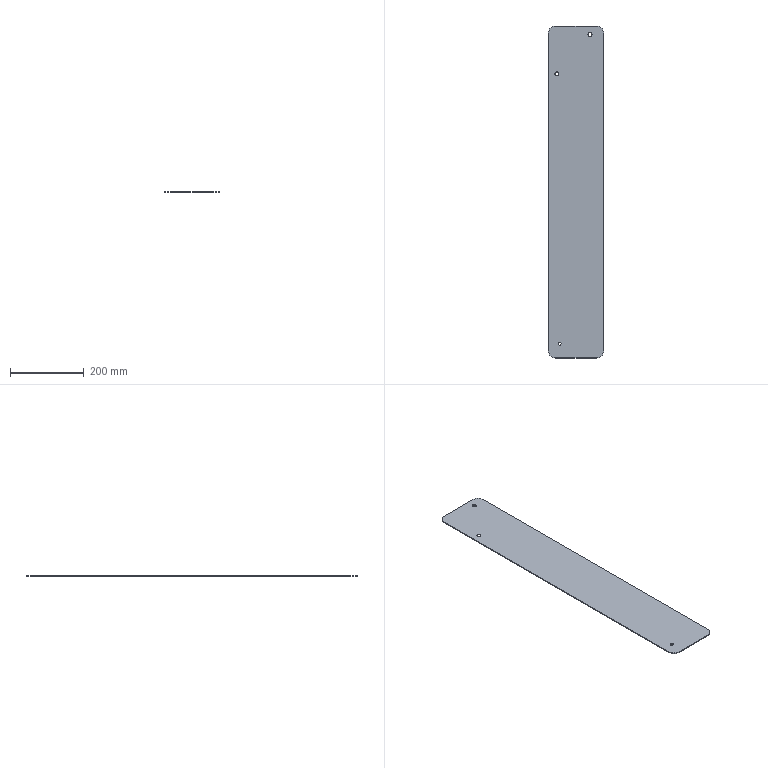Part | SolidWorks | features FlatPattern 1, SMBaseFlange 1, SheetMetal 1 | 1 solid | 16 faces | box 150 x 900 x 2.3 mm | volume 309143 mm3 | cylinder 10 | plane 6 | commonest cylinder face diameters 11 x4 40 x4 8.5 x2
STEP:
#1=CARTESIAN_POINT('',(55.5,-23.,2.3));
#2=VERTEX_POINT('',#1);
#3=CARTESIAN_POINT('',(66.5,-23.,2.3));
#4=VERTEX_POINT('',#3);
#5=CARTESIAN_POINT('',(61.,-23.,2.3));
#6=DIRECTION('',(0.,0.,1.));
#7=DIRECTION('',(1.,0.,0.));
#8=AXIS2_PLACEMENT_3D('',#5,#6,#7);
#9=CIRCLE('',#8,5.5);
#10=EDGE_CURVE('',#2,#4,#9,.T.);
#11=ORIENTED_EDGE('',*,*,#10,.T.);
#12=CARTESIAN_POINT('',(66.5,-23.,0.));
#13=VERTEX_POINT('',#12);
#14=CARTESIAN_POINT('',(66.5,-23.,2.3));
#15=DIRECTION('',(0.,0.,-1.));
#16=VECTOR('',#15,1000.);
#17=LINE('',#14,#16);
#18=EDGE_CURVE('',#4,#13,#17,.T.);
#19=ORIENTED_EDGE('',*,*,#18,.T.);
#20=CARTESIAN_POINT('',(55.5,-23.,0.));
#21=VERTEX_POINT('',#20);
#22=CARTESIAN_POINT('',(61.,-23.,0.));
#23=DIRECTION('',(0.,0.,1.));
#24=DIRECTION('',(1.,0.,0.));
#25=AXIS2_PLACEMENT_3D('',#22,#23,#24);
#26=CIRCLE('',#25,5.5);
#27=EDGE_CURVE('',#21,#13,#26,.T.);
#28=ORIENTED_EDGE('',*,*,#27,.F.);
#29=CARTESIAN_POINT('',(55.5,-23.,2.3));
#30=DIRECTION('',(0.,0.,-1.));
#31=VECTOR('',#30,1000.);
#32=LINE('',#29,#31);
#33=EDGE_CURVE('',#2,#21,#32,.T.);
#34=ORIENTED_EDGE('',*,*,#33,.F.);
#35=EDGE_LOOP('',(#11,#19,#28,#34));
#36=FACE_OUTER_BOUND('',#35,.T.);
#37=CARTESIAN_POINT('',(61.,-23.,2.3));
#38=DIRECTION('',(0.,0.,-1.));
#39=DIRECTION('',(-1.,0.,0.));
#40=AXIS2_PLACEMENT_3D('',#37,#38,#39);
#41=CYLINDRICAL_SURFACE('',#40,5.5);
#42=ADVANCED_FACE('',(#36),#41,.F.);
#43=CARTESIAN_POINT('',(-34.5,-130.,2.3));
#44=VERTEX_POINT('',#43);
#45=CARTESIAN_POINT('',(-23.5,-130.,2.3));
#46=VERTEX_POINT('',#45);
#47=CARTESIAN_POINT('',(-29.,-130.,2.3));
#48=DIRECTION('',(0.,0.,1.));
#49=DIRECTION('',(1.,0.,0.));
#50=AXIS2_PLACEMENT_3D('',#47,#48,#49);
#51=CIRCLE('',#50,5.5);
#52=EDGE_CURVE('',#44,#46,#51,.T.);
#53=ORIENTED_EDGE('',*,*,#52,.T.);
#54=CARTESIAN_POINT('',(-23.5,-130.,0.));
#55=VERTEX_POINT('',#54);
#56=CARTESIAN_POINT('',(-23.5,-130.,2.3));
#57=DIRECTION('',(0.,0.,-1.));
#58=VECTOR('',#57,1000.);
#59=LINE('',#56,#58);
#60=EDGE_CURVE('',#46,#55,#59,.T.);
#61=ORIENTED_EDGE('',*,*,#60,.T.);
#62=CARTESIAN_POINT('',(-34.5,-130.,0.));
#63=VERTEX_POINT('',#62);
#64=CARTESIAN_POINT('',(-29.,-130.,0.));
#65=DIRECTION('',(0.,0.,1.));
#66=DIRECTION('',(1.,0.,0.));
#67=AXIS2_PLACEMENT_3D('',#64,#65,#66);
#68=CIRCLE('',#67,5.5);
#69=EDGE_CURVE('',#63,#55,#68,.T.);
#70=ORIENTED_EDGE('',*,*,#69,.F.);
#71=CARTESIAN_POINT('',(-34.5,-130.,2.3));
#72=DIRECTION('',(0.,0.,-1.));
#73=VECTOR('',#72,1000.);
#74=LINE('',#71,#73);
#75=EDGE_CURVE('',#44,#63,#74,.T.);
#76=ORIENTED_EDGE('',*,*,#75,.F.);
#77=EDGE_LOOP('',(#53,#61,#70,#76));
#78=FACE_OUTER_BOUND('',#77,.T.);
#79=CARTESIAN_POINT('',(-29.,-130.,2.3));
#80=DIRECTION('',(0.,0.,-1.));
#81=DIRECTION('',(-1.,0.,0.));
#82=AXIS2_PLACEMENT_3D('',#79,#80,#81);
#83=CYLINDRICAL_SURFACE('',#82,5.5);
#84=ADVANCED_FACE('',(#78),#83,.F.);
#85=CARTESIAN_POINT('',(-25.75,-861.,2.3));
#86=VERTEX_POINT('',#85);
#87=CARTESIAN_POINT('',(-17.25,-861.,2.3));
#88=VERTEX_POINT('',#87);
#89=CARTESIAN_POINT('',(-21.5,-861.,2.3));
#90=DIRECTION('',(0.,0.,1.));
#91=DIRECTION('',(1.,0.,0.));
#92=AXIS2_PLACEMENT_3D('',#89,#90,#91);
#93=CIRCLE('',#92,4.25);
#94=EDGE_CURVE('',#86,#88,#93,.T.);
#95=ORIENTED_EDGE('',*,*,#94,.T.);
#96=CARTESIAN_POINT('',(-17.25,-861.,0.));
#97=VERTEX_POINT('',#96);
#98=CARTESIAN_POINT('',(-17.25,-861.,2.3));
#99=DIRECTION('',(0.,0.,-1.));
#100=VECTOR('',#99,1000.);
#101=LINE('',#98,#100);
#102=EDGE_CURVE('',#88,#97,#101,.T.);
#103=ORIENTED_EDGE('',*,*,#102,.T.);
#104=CARTESIAN_POINT('',(-25.75,-861.,0.));
#105=VERTEX_POINT('',#104);
#106=CARTESIAN_POINT('',(-21.5,-861.,0.));
#107=DIRECTION('',(0.,0.,1.));
#108=DIRECTION('',(1.,0.,0.));
#109=AXIS2_PLACEMENT_3D('',#106,#107,#108);
#110=CIRCLE('',#109,4.25);
#111=EDGE_CURVE('',#105,#97,#110,.T.);
#112=ORIENTED_EDGE('',*,*,#111,.F.);
#113=CARTESIAN_POINT('',(-25.75,-861.,2.3));
#114=DIRECTION('',(0.,0.,-1.));
#115=VECTOR('',#114,1000.);
#116=LINE('',#113,#115);
#117=EDGE_CURVE('',#86,#105,#116,.T.);
#118=ORIENTED_EDGE('',*,*,#117,.F.);
#119=EDGE_LOOP('',(#95,#103,#112,#118));
#120=FACE_OUTER_BOUND('',#119,.T.);
#121=CARTESIAN_POINT('',(-21.5,-861.,2.3));
#122=DIRECTION('',(0.,0.,-1.));
#123=DIRECTION('',(-1.,0.,0.));
#124=AXIS2_PLACEMENT_3D('',#121,#122,#123);
#125=CYLINDRICAL_SURFACE('',#124,4.25);
#126=ADVANCED_FACE('',(#120),#125,.F.);
#127=CARTESIAN_POINT('',(98.,-20.,2.3));
#128=VERTEX_POINT('',#127);
#129=CARTESIAN_POINT('',(78.,0.,2.3));
#130=VERTEX_POINT('',#129);
#131=CARTESIAN_POINT('',(78.,-20.,2.3));
#132=DIRECTION('',(0.,0.,1.));
#133=DIRECTION('',(-1.,0.,0.));
#134=AXIS2_PLACEMENT_3D('',#131,#132,#133);
#135=CIRCLE('',#134,20.);
#136=EDGE_CURVE('',#128,#130,#135,.T.);
#137=ORIENTED_EDGE('',*,*,#136,.T.);
#138=CARTESIAN_POINT('',(-32.,0.,2.3));
#139=VERTEX_POINT('',#138);
#140=CARTESIAN_POINT('',(-32.,0.,2.3));
#141=DIRECTION('',(-1.,0.,0.));
#142=VECTOR('',#141,1000.);
#143=LINE('',#140,#142);
#144=EDGE_CURVE('',#130,#139,#143,.T.);
#145=ORIENTED_EDGE('',*,*,#144,.T.);
#146=CARTESIAN_POINT('',(-52.,-20.,2.3));
#147=VERTEX_POINT('',#146);
#148=CARTESIAN_POINT('',(-32.,-20.,2.3));
#149=DIRECTION('',(0.,0.,1.));
#150=DIRECTION('',(-1.,0.,0.));
#151=AXIS2_PLACEMENT_3D('',#148,#149,#150);
#152=CIRCLE('',#151,20.);
#153=EDGE_CURVE('',#139,#147,#152,.T.);
#154=ORIENTED_EDGE('',*,*,#153,.T.);
#155=CARTESIAN_POINT('',(-52.,-880.,2.3));
#156=VERTEX_POINT('',#155);
#157=CARTESIAN_POINT('',(-52.,-880.,2.3));
#158=DIRECTION('',(0.,-1.,0.));
#159=VECTOR('',#158,1000.);
#160=LINE('',#157,#159);
#161=EDGE_CURVE('',#147,#156,#160,.T.);
#162=ORIENTED_EDGE('',*,*,#161,.T.);
#163=CARTESIAN_POINT('',(-32.,-900.,2.3));
#164=VERTEX_POINT('',#163);
#165=CARTESIAN_POINT('',(-32.,-880.,2.3));
#166=DIRECTION('',(0.,0.,1.));
#167=DIRECTION('',(-1.,0.,0.));
#168=AXIS2_PLACEMENT_3D('',#165,#166,#167);
#169=CIRCLE('',#168,20.);
#170=EDGE_CURVE('',#156,#164,#169,.T.);
#171=ORIENTED_EDGE('',*,*,#170,.T.);
#172=CARTESIAN_POINT('',(78.,-900.,2.3));
#173=VERTEX_POINT('',#172);
#174=CARTESIAN_POINT('',(-32.,-900.,2.3));
#175=DIRECTION('',(1.,0.,0.));
#176=VECTOR('',#175,1000.);
#177=LINE('',#174,#176);
#178=EDGE_CURVE('',#164,#173,#177,.T.);
#179=ORIENTED_EDGE('',*,*,#178,.T.);
#180=CARTESIAN_POINT('',(98.,-880.,2.3));
#181=VERTEX_POINT('',#180);
#182=CARTESIAN_POINT('',(78.,-880.,2.3));
#183=DIRECTION('',(0.,0.,1.));
#184=DIRECTION('',(1.,0.,0.));
#185=AXIS2_PLACEMENT_3D('',#182,#183,#184);
#186=CIRCLE('',#185,20.);
#187=EDGE_CURVE('',#173,#181,#186,.T.);
#188=ORIENTED_EDGE('',*,*,#187,.T.);
#189=CARTESIAN_POINT('',(98.,-880.,2.3));
#190=DIRECTION('',(0.,1.,0.));
#191=VECTOR('',#190,1000.);
#192=LINE('',#189,#191);
#193=EDGE_CURVE('',#181,#128,#192,.T.);
#194=ORIENTED_EDGE('',*,*,#193,.T.);
#195=EDGE_LOOP('',(#137,#145,#154,#162,#171,#179,#188,#194));
#196=FACE_OUTER_BOUND('',#195,.T.);
#197=ORIENTED_EDGE('',*,*,#94,.F.);
#198=CARTESIAN_POINT('',(-21.5,-861.,2.3));
#199=DIRECTION('',(0.,0.,1.));
#200=DIRECTION('',(1.,0.,0.));
#201=AXIS2_PLACEMENT_3D('',#198,#199,#200);
#202=CIRCLE('',#201,4.25);
#203=EDGE_CURVE('',#88,#86,#202,.T.);
#204=ORIENTED_EDGE('',*,*,#203,.F.);
#205=EDGE_LOOP('',(#197,#204));
#206=FACE_BOUND('',#205,.T.);
#207=ORIENTED_EDGE('',*,*,#52,.F.);
#208=CARTESIAN_POINT('',(-29.,-130.,2.3));
#209=DIRECTION('',(0.,0.,1.));
#210=DIRECTION('',(1.,0.,0.));
#211=AXIS2_PLACEMENT_3D('',#208,#209,#210);
#212=CIRCLE('',#211,5.5);
#213=EDGE_CURVE('',#46,#44,#212,.T.);
#214=ORIENTED_EDGE('',*,*,#213,.F.);
#215=EDGE_LOOP('',(#207,#214));
#216=FACE_BOUND('',#215,.T.);
#217=ORIENTED_EDGE('',*,*,#10,.F.);
#218=CARTESIAN_POINT('',(61.,-23.,2.3));
#219=DIRECTION('',(0.,0.,1.));
#220=DIRECTION('',(1.,0.,0.));
#221=AXIS2_PLACEMENT_3D('',#218,#219,#220);
#222=CIRCLE('',#221,5.5);
#223=EDGE_CURVE('',#4,#2,#222,.T.);
#224=ORIENTED_EDGE('',*,*,#223,.F.);
#225=EDGE_LOOP('',(#217,#224));
#226=FACE_BOUND('',#225,.T.);
#227=CARTESIAN_POINT('',(78.,-20.,2.3));
#228=DIRECTION('',(0.,0.,-1.));
#229=DIRECTION('',(-1.,0.,0.));
#230=AXIS2_PLACEMENT_3D('',#227,#228,#229);
#231=PLANE('',#230);
#232=ADVANCED_FACE('',(#196,#206,#216,#226),#231,.F.);
#233=ORIENTED_EDGE('',*,*,#69,.T.);
#234=CARTESIAN_POINT('',(-29.,-130.,0.));
#235=DIRECTION('',(0.,0.,1.));
#236=DIRECTION('',(1.,0.,0.));
#237=AXIS2_PLACEMENT_3D('',#234,#235,#236);
#238=CIRCLE('',#237,5.5);
#239=EDGE_CURVE('',#55,#63,#238,.T.);
#240=ORIENTED_EDGE('',*,*,#239,.T.);
#241=EDGE_LOOP('',(#233,#240));
#242=FACE_BOUND('',#241,.T.);
#243=CARTESIAN_POINT('',(98.,-20.,0.));
#244=VERTEX_POINT('',#243);
#245=CARTESIAN_POINT('',(78.,0.,0.));
#246=VERTEX_POINT('',#245);
#247=CARTESIAN_POINT('',(78.,-20.,0.));
#248=DIRECTION('',(0.,0.,1.));
#249=DIRECTION('',(-1.,0.,0.));
#250=AXIS2_PLACEMENT_3D('',#247,#248,#249);
#251=CIRCLE('',#250,20.);
#252=EDGE_CURVE('',#244,#246,#251,.T.);
#253=ORIENTED_EDGE('',*,*,#252,.F.);
#254=CARTESIAN_POINT('',(98.,-880.,0.));
#255=VERTEX_POINT('',#254);
#256=CARTESIAN_POINT('',(98.,-880.,0.));
#257=DIRECTION('',(0.,1.,0.));
#258=VECTOR('',#257,1000.);
#259=LINE('',#256,#258);
#260=EDGE_CURVE('',#255,#244,#259,.T.);
#261=ORIENTED_EDGE('',*,*,#260,.F.);
#262=CARTESIAN_POINT('',(78.,-900.,0.));
#263=VERTEX_POINT('',#262);
#264=CARTESIAN_POINT('',(78.,-880.,0.));
#265=DIRECTION('',(0.,0.,1.));
#266=DIRECTION('',(1.,0.,0.));
#267=AXIS2_PLACEMENT_3D('',#264,#265,#266);
#268=CIRCLE('',#267,20.);
#269=EDGE_CURVE('',#263,#255,#268,.T.);
#270=ORIENTED_EDGE('',*,*,#269,.F.);
#271=CARTESIAN_POINT('',(-32.,-900.,0.));
#272=VERTEX_POINT('',#271);
#273=CARTESIAN_POINT('',(-32.,-900.,0.));
#274=DIRECTION('',(1.,0.,0.));
#275=VECTOR('',#274,1000.);
#276=LINE('',#273,#275);
#277=EDGE_CURVE('',#272,#263,#276,.T.);
#278=ORIENTED_EDGE('',*,*,#277,.F.);
#279=CARTESIAN_POINT('',(-52.,-880.,0.));
#280=VERTEX_POINT('',#279);
#281=CARTESIAN_POINT('',(-32.,-880.,0.));
#282=DIRECTION('',(0.,0.,1.));
#283=DIRECTION('',(-1.,0.,0.));
#284=AXIS2_PLACEMENT_3D('',#281,#282,#283);
#285=CIRCLE('',#284,20.);
#286=EDGE_CURVE('',#280,#272,#285,.T.);
#287=ORIENTED_EDGE('',*,*,#286,.F.);
#288=CARTESIAN_POINT('',(-52.,-20.,0.));
#289=VERTEX_POINT('',#288);
#290=CARTESIAN_POINT('',(-52.,-880.,0.));
#291=DIRECTION('',(0.,-1.,0.));
#292=VECTOR('',#291,1000.);
#293=LINE('',#290,#292);
#294=EDGE_CURVE('',#289,#280,#293,.T.);
#295=ORIENTED_EDGE('',*,*,#294,.F.);
#296=CARTESIAN_POINT('',(-32.,0.,0.));
#297=VERTEX_POINT('',#296);
#298=CARTESIAN_POINT('',(-32.,-20.,0.));
#299=DIRECTION('',(0.,0.,1.));
#300=DIRECTION('',(-1.,0.,0.));
#301=AXIS2_PLACEMENT_3D('',#298,#299,#300);
#302=CIRCLE('',#301,20.);
#303=EDGE_CURVE('',#297,#289,#302,.T.);
#304=ORIENTED_EDGE('',*,*,#303,.F.);
#305=CARTESIAN_POINT('',(-32.,0.,0.));
#306=DIRECTION('',(-1.,0.,0.));
#307=VECTOR('',#306,1000.);
#308=LINE('',#305,#307);
#309=EDGE_CURVE('',#246,#297,#308,.T.);
#310=ORIENTED_EDGE('',*,*,#309,.F.);
#311=EDGE_LOOP('',(#253,#261,#270,#278,#287,#295,#304,#310));
#312=FACE_OUTER_BOUND('',#311,.T.);
#313=ORIENTED_EDGE('',*,*,#111,.T.);
#314=CARTESIAN_POINT('',(-21.5,-861.,0.));
#315=DIRECTION('',(0.,0.,1.));
#316=DIRECTION('',(1.,0.,0.));
#317=AXIS2_PLACEMENT_3D('',#314,#315,#316);
#318=CIRCLE('',#317,4.25);
#319=EDGE_CURVE('',#97,#105,#318,.T.);
#320=ORIENTED_EDGE('',*,*,#319,.T.);
#321=EDGE_LOOP('',(#313,#320));
#322=FACE_BOUND('',#321,.T.);
#323=ORIENTED_EDGE('',*,*,#27,.T.);
#324=CARTESIAN_POINT('',(61.,-23.,0.));
#325=DIRECTION('',(0.,0.,1.));
#326=DIRECTION('',(1.,0.,0.));
#327=AXIS2_PLACEMENT_3D('',#324,#325,#326);
#328=CIRCLE('',#327,5.5);
#329=EDGE_CURVE('',#13,#21,#328,.T.);
#330=ORIENTED_EDGE('',*,*,#329,.T.);
#331=EDGE_LOOP('',(#323,#330));
#332=FACE_BOUND('',#331,.T.);
#333=CARTESIAN_POINT('',(78.,-20.,0.));
#334=DIRECTION('',(0.,0.,-1.));
#335=DIRECTION('',(-1.,0.,0.));
#336=AXIS2_PLACEMENT_3D('',#333,#334,#335);
#337=PLANE('',#336);
#338=ADVANCED_FACE('',(#242,#312,#322,#332),#337,.T.);
#339=ORIENTED_EDGE('',*,*,#252,.T.);
#340=CARTESIAN_POINT('',(78.,0.,2.3));
#341=DIRECTION('',(0.,0.,-1.));
#342=VECTOR('',#341,1000.);
#343=LINE('',#340,#342);
#344=EDGE_CURVE('',#130,#246,#343,.T.);
#345=ORIENTED_EDGE('',*,*,#344,.F.);
#346=ORIENTED_EDGE('',*,*,#136,.F.);
#347=CARTESIAN_POINT('',(98.,-20.,2.3));
#348=DIRECTION('',(0.,0.,-1.));
#349=VECTOR('',#348,1000.);
#350=LINE('',#347,#349);
#351=EDGE_CURVE('',#128,#244,#350,.T.);
#352=ORIENTED_EDGE('',*,*,#351,.T.);
#353=EDGE_LOOP('',(#339,#345,#346,#352));
#354=FACE_OUTER_BOUND('',#353,.T.);
#355=CARTESIAN_POINT('',(78.,-20.,2.3));
#356=DIRECTION('',(0.,0.,-1.));
#357=DIRECTION('',(-1.,0.,0.));
#358=AXIS2_PLACEMENT_3D('',#355,#356,#357);
#359=CYLINDRICAL_SURFACE('',#358,20.);
#360=ADVANCED_FACE('',(#354),#359,.T.);
#361=ORIENTED_EDGE('',*,*,#309,.T.);
#362=CARTESIAN_POINT('',(-32.,0.,2.3));
#363=DIRECTION('',(0.,0.,-1.));
#364=VECTOR('',#363,1000.);
#365=LINE('',#362,#364);
#366=EDGE_CURVE('',#139,#297,#365,.T.);
#367=ORIENTED_EDGE('',*,*,#366,.F.);
#368=ORIENTED_EDGE('',*,*,#144,.F.);
#369=ORIENTED_EDGE('',*,*,#344,.T.);
#370=EDGE_LOOP('',(#361,#367,#368,#369));
#371=FACE_OUTER_BOUND('',#370,.T.);
#372=CARTESIAN_POINT('',(-32.,0.,2.3));
#373=DIRECTION('',(0.,-1.,0.));
#374=DIRECTION('',(0.,0.,-1.));
#375=AXIS2_PLACEMENT_3D('',#372,#373,#374);
#376=PLANE('',#375);
#377=ADVANCED_FACE('',(#371),#376,.F.);
#378=ORIENTED_EDGE('',*,*,#303,.T.);
#379=CARTESIAN_POINT('',(-52.,-20.,2.3));
#380=DIRECTION('',(0.,0.,-1.));
#381=VECTOR('',#380,1000.);
#382=LINE('',#379,#381);
#383=EDGE_CURVE('',#147,#289,#382,.T.);
#384=ORIENTED_EDGE('',*,*,#383,.F.);
#385=ORIENTED_EDGE('',*,*,#153,.F.);
#386=ORIENTED_EDGE('',*,*,#366,.T.);
#387=EDGE_LOOP('',(#378,#384,#385,#386));
#388=FACE_OUTER_BOUND('',#387,.T.);
#389=CARTESIAN_POINT('',(-32.,-20.,2.3));
#390=DIRECTION('',(0.,0.,-1.));
#391=DIRECTION('',(-1.,0.,0.));
#392=AXIS2_PLACEMENT_3D('',#389,#390,#391);
#393=CYLINDRICAL_SURFACE('',#392,20.);
#394=ADVANCED_FACE('',(#388),#393,.T.);
#395=ORIENTED_EDGE('',*,*,#294,.T.);
#396=CARTESIAN_POINT('',(-52.,-880.,2.3));
#397=DIRECTION('',(0.,0.,-1.));
#398=VECTOR('',#397,1000.);
#399=LINE('',#396,#398);
#400=EDGE_CURVE('',#156,#280,#399,.T.);
#401=ORIENTED_EDGE('',*,*,#400,.F.);
#402=ORIENTED_EDGE('',*,*,#161,.F.);
#403=ORIENTED_EDGE('',*,*,#383,.T.);
#404=EDGE_LOOP('',(#395,#401,#402,#403));
#405=FACE_OUTER_BOUND('',#404,.T.);
#406=CARTESIAN_POINT('',(-52.,-880.,2.3));
#407=DIRECTION('',(1.,0.,0.));
#408=DIRECTION('',(0.,0.,-1.));
#409=AXIS2_PLACEMENT_3D('',#406,#407,#408);
#410=PLANE('',#409);
#411=ADVANCED_FACE('',(#405),#410,.F.);
#412=ORIENTED_EDGE('',*,*,#286,.T.);
#413=CARTESIAN_POINT('',(-32.,-900.,2.3));
#414=DIRECTION('',(0.,0.,-1.));
#415=VECTOR('',#414,1000.);
#416=LINE('',#413,#415);
#417=EDGE_CURVE('',#164,#272,#416,.T.);
#418=ORIENTED_EDGE('',*,*,#417,.F.);
#419=ORIENTED_EDGE('',*,*,#170,.F.);
#420=ORIENTED_EDGE('',*,*,#400,.T.);
#421=EDGE_LOOP('',(#412,#418,#419,#420));
#422=FACE_OUTER_BOUND('',#421,.T.);
#423=CARTESIAN_POINT('',(-32.,-880.,2.3));
#424=DIRECTION('',(0.,0.,-1.));
#425=DIRECTION('',(-1.,0.,0.));
#426=AXIS2_PLACEMENT_3D('',#423,#424,#425);
#427=CYLINDRICAL_SURFACE('',#426,20.);
#428=ADVANCED_FACE('',(#422),#427,.T.);
#429=ORIENTED_EDGE('',*,*,#277,.T.);
#430=CARTESIAN_POINT('',(78.,-900.,2.3));
#431=DIRECTION('',(0.,0.,-1.));
#432=VECTOR('',#431,1000.);
#433=LINE('',#430,#432);
#434=EDGE_CURVE('',#173,#263,#433,.T.);
#435=ORIENTED_EDGE('',*,*,#434,.F.);
#436=ORIENTED_EDGE('',*,*,#178,.F.);
#437=ORIENTED_EDGE('',*,*,#417,.T.);
#438=EDGE_LOOP('',(#429,#435,#436,#437));
#439=FACE_OUTER_BOUND('',#438,.T.);
#440=CARTESIAN_POINT('',(-32.,-900.,2.3));
#441=DIRECTION('',(0.,1.,0.));
#442=DIRECTION('',(0.,0.,1.));
#443=AXIS2_PLACEMENT_3D('',#440,#441,#442);
#444=PLANE('',#443);
#445=ADVANCED_FACE('',(#439),#444,.F.);
#446=ORIENTED_EDGE('',*,*,#269,.T.);
#447=CARTESIAN_POINT('',(98.,-880.,2.3));
#448=DIRECTION('',(0.,0.,-1.));
#449=VECTOR('',#448,1000.);
#450=LINE('',#447,#449);
#451=EDGE_CURVE('',#181,#255,#450,.T.);
#452=ORIENTED_EDGE('',*,*,#451,.F.);
#453=ORIENTED_EDGE('',*,*,#187,.F.);
#454=ORIENTED_EDGE('',*,*,#434,.T.);
#455=EDGE_LOOP('',(#446,#452,#453,#454));
#456=FACE_OUTER_BOUND('',#455,.T.);
#457=CARTESIAN_POINT('',(78.,-880.,2.3));
#458=DIRECTION('',(0.,0.,-1.));
#459=DIRECTION('',(-1.,0.,0.));
#460=AXIS2_PLACEMENT_3D('',#457,#458,#459);
#461=CYLINDRICAL_SURFACE('',#460,20.);
#462=ADVANCED_FACE('',(#456),#461,.T.);
#463=ORIENTED_EDGE('',*,*,#260,.T.);
#464=ORIENTED_EDGE('',*,*,#351,.F.);
#465=ORIENTED_EDGE('',*,*,#193,.F.);
#466=ORIENTED_EDGE('',*,*,#451,.T.);
#467=EDGE_LOOP('',(#463,#464,#465,#466));
#468=FACE_OUTER_BOUND('',#467,.T.);
#469=CARTESIAN_POINT('',(98.,-880.,2.3));
#470=DIRECTION('',(-1.,0.,0.));
#471=DIRECTION('',(0.,0.,1.));
#472=AXIS2_PLACEMENT_3D('',#469,#470,#471);
#473=PLANE('',#472);
#474=ADVANCED_FACE('',(#468),#473,.F.);
#475=ORIENTED_EDGE('',*,*,#102,.F.);
#476=ORIENTED_EDGE('',*,*,#203,.T.);
#477=ORIENTED_EDGE('',*,*,#117,.T.);
#478=ORIENTED_EDGE('',*,*,#319,.F.);
#479=EDGE_LOOP('',(#475,#476,#477,#478));
#480=FACE_OUTER_BOUND('',#479,.T.);
#481=CARTESIAN_POINT('',(-21.5,-861.,2.3));
#482=DIRECTION('',(0.,0.,-1.));
#483=DIRECTION('',(-1.,0.,0.));
#484=AXIS2_PLACEMENT_3D('',#481,#482,#483);
#485=CYLINDRICAL_SURFACE('',#484,4.25);
#486=ADVANCED_FACE('',(#480),#485,.F.);
#487=ORIENTED_EDGE('',*,*,#60,.F.);
#488=ORIENTED_EDGE('',*,*,#213,.T.);
#489=ORIENTED_EDGE('',*,*,#75,.T.);
#490=ORIENTED_EDGE('',*,*,#239,.F.);
#491=EDGE_LOOP('',(#487,#488,#489,#490));
#492=FACE_OUTER_BOUND('',#491,.T.);
#493=CARTESIAN_POINT('',(-29.,-130.,2.3));
#494=DIRECTION('',(0.,0.,-1.));
#495=DIRECTION('',(-1.,0.,0.));
#496=AXIS2_PLACEMENT_3D('',#493,#494,#495);
#497=CYLINDRICAL_SURFACE('',#496,5.5);
#498=ADVANCED_FACE('',(#492),#497,.F.);
#499=ORIENTED_EDGE('',*,*,#18,.F.);
#500=ORIENTED_EDGE('',*,*,#223,.T.);
#501=ORIENTED_EDGE('',*,*,#33,.T.);
#502=ORIENTED_EDGE('',*,*,#329,.F.);
#503=EDGE_LOOP('',(#499,#500,#501,#502));
#504=FACE_OUTER_BOUND('',#503,.T.);
#505=CARTESIAN_POINT('',(61.,-23.,2.3));
#506=DIRECTION('',(0.,0.,-1.));
#507=DIRECTION('',(-1.,0.,0.));
#508=AXIS2_PLACEMENT_3D('',#505,#506,#507);
#509=CYLINDRICAL_SURFACE('',#508,5.5);
#510=ADVANCED_FACE('',(#504),#509,.F.);
#511=CLOSED_SHELL('',(#42,#84,#126,#232,#338,#360,#377,#394,#411,#428,#445,#462,#474,#486,#498,#510));
#512=MANIFOLD_SOLID_BREP('',#511);
#513=CARTESIAN_POINT('',(0.,0.,0.));
#514=DIRECTION('',(0.,0.,1.));
#515=DIRECTION('',(1.,0.,0.));
#516=AXIS2_PLACEMENT_3D('',#513,#514,#515);
#517=(LENGTH_UNIT()NAMED_UNIT(*)SI_UNIT(.MILLI.,.METRE.));
#518=UNCERTAINTY_MEASURE_WITH_UNIT(LENGTH_MEASURE(0.00001),#517,'','');
#519=(NAMED_UNIT(*)PLANE_ANGLE_UNIT()SI_UNIT($,.RADIAN.));
#520=(NAMED_UNIT(*)SI_UNIT($,.STERADIAN.)SOLID_ANGLE_UNIT());
#521=(GEOMETRIC_REPRESENTATION_CONTEXT(3)GLOBAL_UNCERTAINTY_ASSIGNED_CONTEXT((#518))GLOBAL_UNIT_ASSIGNED_CONTEXT((#517,#519,#520))REPRESENTATION_CONTEXT('',''));
#522=ADVANCED_BREP_SHAPE_REPRESENTATION('',(#512,#516),#521);